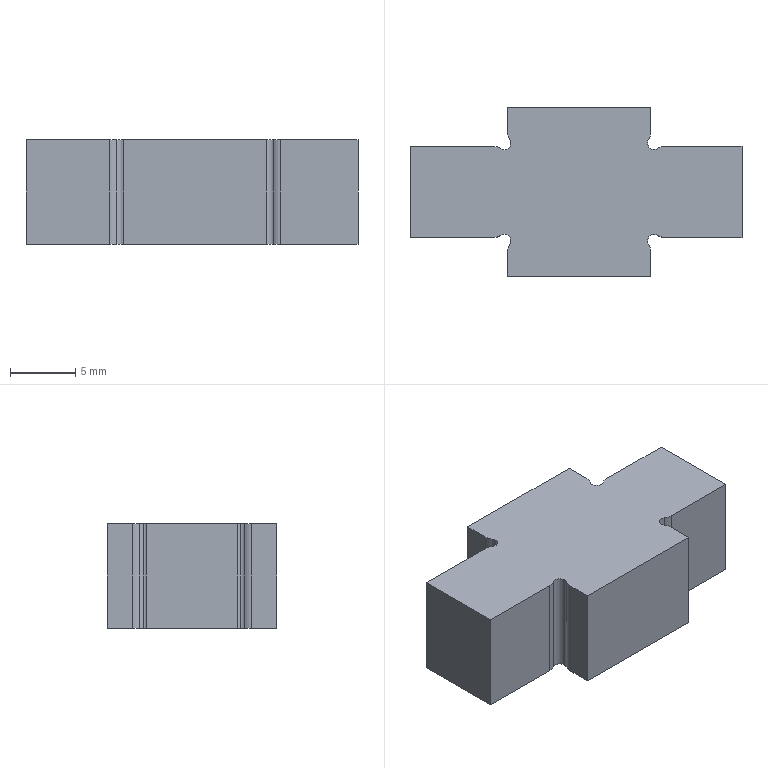Part | SolidWorks | features Fillet 1, FlatPattern 1, ICE 1, SMBaseFlange 1, SheetMetal 1 | 1 solid | 28 faces | box 25.5 x 13 x 8 mm | volume 1946 mm3 | cylinder 14 | plane 14 | commonest cylinder face diameters 2 x8 1 x6
STEP:
#1=CARTESIAN_POINT('',(-6.25,26.293,0.));
#2=VERTEX_POINT('',#1);
#3=CARTESIAN_POINT('',(-6.333,26.569,0.));
#4=VERTEX_POINT('',#3);
#5=CARTESIAN_POINT('',(-6.75,26.293,0.));
#6=DIRECTION('',(0.,0.,1.));
#7=DIRECTION('',(1.,0.,0.));
#8=AXIS2_PLACEMENT_3D('',#5,#6,#7);
#9=CIRCLE('',#8,0.5);
#10=EDGE_CURVE('',#2,#4,#9,.T.);
#11=ORIENTED_EDGE('',*,*,#10,.F.);
#12=CARTESIAN_POINT('',(-6.25,26.293,8.));
#13=VERTEX_POINT('',#12);
#14=CARTESIAN_POINT('',(-6.25,26.293,0.));
#15=DIRECTION('',(0.,0.,1.));
#16=VECTOR('',#15,1000.);
#17=LINE('',#14,#16);
#18=EDGE_CURVE('',#2,#13,#17,.T.);
#19=ORIENTED_EDGE('',*,*,#18,.T.);
#20=CARTESIAN_POINT('',(-6.333,26.569,8.));
#21=VERTEX_POINT('',#20);
#22=CARTESIAN_POINT('',(-6.75,26.293,8.));
#23=DIRECTION('',(0.,0.,1.));
#24=DIRECTION('',(1.,0.,0.));
#25=AXIS2_PLACEMENT_3D('',#22,#23,#24);
#26=CIRCLE('',#25,0.5);
#27=EDGE_CURVE('',#13,#21,#26,.T.);
#28=ORIENTED_EDGE('',*,*,#27,.T.);
#29=CARTESIAN_POINT('',(-6.333,26.569,0.));
#30=DIRECTION('',(0.,0.,-1.));
#31=VECTOR('',#30,1000.);
#32=LINE('',#29,#31);
#33=EDGE_CURVE('',#21,#4,#32,.T.);
#34=ORIENTED_EDGE('',*,*,#33,.T.);
#35=EDGE_LOOP('',(#11,#19,#28,#34));
#36=FACE_OUTER_BOUND('',#35,.T.);
#37=CARTESIAN_POINT('',(-6.75,26.293,0.));
#38=DIRECTION('',(0.,0.,1.));
#39=DIRECTION('',(1.,0.,0.));
#40=AXIS2_PLACEMENT_3D('',#37,#38,#39);
#41=CYLINDRICAL_SURFACE('',#40,0.5);
#42=ADVANCED_FACE('',(#36),#41,.F.);
#43=CARTESIAN_POINT('',(-6.25,18.793,0.));
#44=VERTEX_POINT('',#43);
#45=CARTESIAN_POINT('',(-7.026,19.209,0.));
#46=VERTEX_POINT('',#45);
#47=CARTESIAN_POINT('',(-6.75,18.793,0.));
#48=DIRECTION('',(0.,0.,1.));
#49=DIRECTION('',(1.,0.,0.));
#50=AXIS2_PLACEMENT_3D('',#47,#48,#49);
#51=CIRCLE('',#50,0.5);
#52=EDGE_CURVE('',#44,#46,#51,.T.);
#53=ORIENTED_EDGE('',*,*,#52,.F.);
#54=CARTESIAN_POINT('',(-6.25,18.793,8.));
#55=VERTEX_POINT('',#54);
#56=CARTESIAN_POINT('',(-6.25,18.793,8.));
#57=DIRECTION('',(0.,0.,1.));
#58=VECTOR('',#57,1000.);
#59=LINE('',#56,#58);
#60=EDGE_CURVE('',#44,#55,#59,.T.);
#61=ORIENTED_EDGE('',*,*,#60,.T.);
#62=CARTESIAN_POINT('',(-7.026,19.209,8.));
#63=VERTEX_POINT('',#62);
#64=CARTESIAN_POINT('',(-6.75,18.793,8.));
#65=DIRECTION('',(0.,0.,1.));
#66=DIRECTION('',(1.,0.,0.));
#67=AXIS2_PLACEMENT_3D('',#64,#65,#66);
#68=CIRCLE('',#67,0.5);
#69=EDGE_CURVE('',#55,#63,#68,.T.);
#70=ORIENTED_EDGE('',*,*,#69,.T.);
#71=CARTESIAN_POINT('',(-7.026,19.209,8.));
#72=DIRECTION('',(0.,0.,-1.));
#73=VECTOR('',#72,1000.);
#74=LINE('',#71,#73);
#75=EDGE_CURVE('',#63,#46,#74,.T.);
#76=ORIENTED_EDGE('',*,*,#75,.T.);
#77=EDGE_LOOP('',(#53,#61,#70,#76));
#78=FACE_OUTER_BOUND('',#77,.T.);
#79=CARTESIAN_POINT('',(-6.75,18.793,8.));
#80=DIRECTION('',(0.,0.,1.));
#81=DIRECTION('',(1.,0.,0.));
#82=AXIS2_PLACEMENT_3D('',#79,#80,#81);
#83=CYLINDRICAL_SURFACE('',#82,0.5);
#84=ADVANCED_FACE('',(#78),#83,.F.);
#85=CARTESIAN_POINT('',(-6.5,17.963,8.));
#86=VERTEX_POINT('',#85);
#87=CARTESIAN_POINT('',(-6.5,16.043,8.));
#88=VERTEX_POINT('',#87);
#89=CARTESIAN_POINT('',(-6.5,19.043,8.));
#90=DIRECTION('',(0.,-1.,0.));
#91=VECTOR('',#90,1000.);
#92=LINE('',#89,#91);
#93=EDGE_CURVE('',#86,#88,#92,.T.);
#94=ORIENTED_EDGE('',*,*,#93,.F.);
#95=CARTESIAN_POINT('',(-6.5,17.963,0.));
#96=VERTEX_POINT('',#95);
#97=CARTESIAN_POINT('',(-6.5,17.963,0.));
#98=DIRECTION('',(0.,0.,-1.));
#99=VECTOR('',#98,1000.);
#100=LINE('',#97,#99);
#101=EDGE_CURVE('',#86,#96,#100,.T.);
#102=ORIENTED_EDGE('',*,*,#101,.T.);
#103=CARTESIAN_POINT('',(-6.5,16.043,0.));
#104=VERTEX_POINT('',#103);
#105=CARTESIAN_POINT('',(-6.5,19.043,0.));
#106=DIRECTION('',(0.,-1.,0.));
#107=VECTOR('',#106,1000.);
#108=LINE('',#105,#107);
#109=EDGE_CURVE('',#96,#104,#108,.T.);
#110=ORIENTED_EDGE('',*,*,#109,.T.);
#111=CARTESIAN_POINT('',(-6.5,16.043,8.));
#112=DIRECTION('',(0.,0.,-1.));
#113=VECTOR('',#112,1000.);
#114=LINE('',#111,#113);
#115=EDGE_CURVE('',#88,#104,#114,.T.);
#116=ORIENTED_EDGE('',*,*,#115,.F.);
#117=EDGE_LOOP('',(#94,#102,#110,#116));
#118=FACE_OUTER_BOUND('',#117,.T.);
#119=CARTESIAN_POINT('',(-6.5,19.043,8.));
#120=DIRECTION('',(1.,0.,0.));
#121=DIRECTION('',(0.,1.,0.));
#122=AXIS2_PLACEMENT_3D('',#119,#120,#121);
#123=PLANE('',#122);
#124=ADVANCED_FACE('',(#118),#123,.F.);
#125=CARTESIAN_POINT('',(4.5,16.043,0.));
#126=VERTEX_POINT('',#125);
#127=CARTESIAN_POINT('',(4.5,17.963,0.));
#128=VERTEX_POINT('',#127);
#129=CARTESIAN_POINT('',(4.5,16.043,0.));
#130=DIRECTION('',(0.,1.,0.));
#131=VECTOR('',#130,1000.);
#132=LINE('',#129,#131);
#133=EDGE_CURVE('',#126,#128,#132,.T.);
#134=ORIENTED_EDGE('',*,*,#133,.T.);
#135=CARTESIAN_POINT('',(4.5,17.963,8.));
#136=VERTEX_POINT('',#135);
#137=CARTESIAN_POINT('',(4.5,17.963,8.));
#138=DIRECTION('',(0.,0.,1.));
#139=VECTOR('',#138,1000.);
#140=LINE('',#137,#139);
#141=EDGE_CURVE('',#128,#136,#140,.T.);
#142=ORIENTED_EDGE('',*,*,#141,.T.);
#143=CARTESIAN_POINT('',(4.5,16.043,8.));
#144=VERTEX_POINT('',#143);
#145=CARTESIAN_POINT('',(4.5,16.043,8.));
#146=DIRECTION('',(0.,1.,0.));
#147=VECTOR('',#146,1000.);
#148=LINE('',#145,#147);
#149=EDGE_CURVE('',#144,#136,#148,.T.);
#150=ORIENTED_EDGE('',*,*,#149,.F.);
#151=CARTESIAN_POINT('',(4.5,16.043,8.));
#152=DIRECTION('',(0.,0.,-1.));
#153=VECTOR('',#152,1000.);
#154=LINE('',#151,#153);
#155=EDGE_CURVE('',#144,#126,#154,.T.);
#156=ORIENTED_EDGE('',*,*,#155,.T.);
#157=EDGE_LOOP('',(#134,#142,#150,#156));
#158=FACE_OUTER_BOUND('',#157,.T.);
#159=CARTESIAN_POINT('',(4.5,16.043,8.));
#160=DIRECTION('',(-1.,0.,0.));
#161=DIRECTION('',(0.,0.,1.));
#162=AXIS2_PLACEMENT_3D('',#159,#160,#161);
#163=PLANE('',#162);
#164=ADVANCED_FACE('',(#158),#163,.F.);
#165=CARTESIAN_POINT('',(5.579,19.043,8.));
#166=VERTEX_POINT('',#165);
#167=CARTESIAN_POINT('',(11.5,19.043,8.));
#168=VERTEX_POINT('',#167);
#169=CARTESIAN_POINT('',(4.5,19.043,8.));
#170=DIRECTION('',(1.,0.,0.));
#171=VECTOR('',#170,1000.);
#172=LINE('',#169,#171);
#173=EDGE_CURVE('',#166,#168,#172,.T.);
#174=ORIENTED_EDGE('',*,*,#173,.F.);
#175=CARTESIAN_POINT('',(5.579,19.043,0.));
#176=VERTEX_POINT('',#175);
#177=CARTESIAN_POINT('',(5.579,19.043,0.));
#178=DIRECTION('',(0.,0.,-1.));
#179=VECTOR('',#178,1000.);
#180=LINE('',#177,#179);
#181=EDGE_CURVE('',#166,#176,#180,.T.);
#182=ORIENTED_EDGE('',*,*,#181,.T.);
#183=CARTESIAN_POINT('',(11.5,19.043,0.));
#184=VERTEX_POINT('',#183);
#185=CARTESIAN_POINT('',(4.5,19.043,0.));
#186=DIRECTION('',(1.,0.,0.));
#187=VECTOR('',#186,1000.);
#188=LINE('',#185,#187);
#189=EDGE_CURVE('',#176,#184,#188,.T.);
#190=ORIENTED_EDGE('',*,*,#189,.T.);
#191=CARTESIAN_POINT('',(11.5,19.043,8.));
#192=DIRECTION('',(0.,0.,-1.));
#193=VECTOR('',#192,1000.);
#194=LINE('',#191,#193);
#195=EDGE_CURVE('',#168,#184,#194,.T.);
#196=ORIENTED_EDGE('',*,*,#195,.F.);
#197=EDGE_LOOP('',(#174,#182,#190,#196));
#198=FACE_OUTER_BOUND('',#197,.T.);
#199=CARTESIAN_POINT('',(4.5,19.043,8.));
#200=DIRECTION('',(0.,1.,0.));
#201=DIRECTION('',(0.,0.,1.));
#202=AXIS2_PLACEMENT_3D('',#199,#200,#201);
#203=PLANE('',#202);
#204=ADVANCED_FACE('',(#198),#203,.F.);
#205=CARTESIAN_POINT('',(11.5,26.043,0.));
#206=VERTEX_POINT('',#205);
#207=CARTESIAN_POINT('',(5.579,26.043,0.));
#208=VERTEX_POINT('',#207);
#209=CARTESIAN_POINT('',(11.5,26.043,0.));
#210=DIRECTION('',(-1.,0.,0.));
#211=VECTOR('',#210,1000.);
#212=LINE('',#209,#211);
#213=EDGE_CURVE('',#206,#208,#212,.T.);
#214=ORIENTED_EDGE('',*,*,#213,.T.);
#215=CARTESIAN_POINT('',(5.579,26.043,8.));
#216=VERTEX_POINT('',#215);
#217=CARTESIAN_POINT('',(5.579,26.043,8.));
#218=DIRECTION('',(0.,0.,1.));
#219=VECTOR('',#218,1000.);
#220=LINE('',#217,#219);
#221=EDGE_CURVE('',#208,#216,#220,.T.);
#222=ORIENTED_EDGE('',*,*,#221,.T.);
#223=CARTESIAN_POINT('',(11.5,26.043,8.));
#224=VERTEX_POINT('',#223);
#225=CARTESIAN_POINT('',(11.5,26.043,8.));
#226=DIRECTION('',(-1.,0.,0.));
#227=VECTOR('',#226,1000.);
#228=LINE('',#225,#227);
#229=EDGE_CURVE('',#224,#216,#228,.T.);
#230=ORIENTED_EDGE('',*,*,#229,.F.);
#231=CARTESIAN_POINT('',(11.5,26.043,8.));
#232=DIRECTION('',(0.,0.,-1.));
#233=VECTOR('',#232,1000.);
#234=LINE('',#231,#233);
#235=EDGE_CURVE('',#224,#206,#234,.T.);
#236=ORIENTED_EDGE('',*,*,#235,.T.);
#237=EDGE_LOOP('',(#214,#222,#230,#236));
#238=FACE_OUTER_BOUND('',#237,.T.);
#239=CARTESIAN_POINT('',(11.5,26.043,8.));
#240=DIRECTION('',(0.,-1.,0.));
#241=DIRECTION('',(0.,0.,-1.));
#242=AXIS2_PLACEMENT_3D('',#239,#240,#241);
#243=PLANE('',#242);
#244=ADVANCED_FACE('',(#238),#243,.F.);
#245=CARTESIAN_POINT('',(4.5,27.122,8.));
#246=VERTEX_POINT('',#245);
#247=CARTESIAN_POINT('',(4.5,29.043,8.));
#248=VERTEX_POINT('',#247);
#249=CARTESIAN_POINT('',(4.5,26.043,8.));
#250=DIRECTION('',(0.,1.,0.));
#251=VECTOR('',#250,1000.);
#252=LINE('',#249,#251);
#253=EDGE_CURVE('',#246,#248,#252,.T.);
#254=ORIENTED_EDGE('',*,*,#253,.F.);
#255=CARTESIAN_POINT('',(4.5,27.122,0.));
#256=VERTEX_POINT('',#255);
#257=CARTESIAN_POINT('',(4.5,27.122,0.));
#258=DIRECTION('',(0.,0.,-1.));
#259=VECTOR('',#258,1000.);
#260=LINE('',#257,#259);
#261=EDGE_CURVE('',#246,#256,#260,.T.);
#262=ORIENTED_EDGE('',*,*,#261,.T.);
#263=CARTESIAN_POINT('',(4.5,29.043,0.));
#264=VERTEX_POINT('',#263);
#265=CARTESIAN_POINT('',(4.5,26.043,0.));
#266=DIRECTION('',(0.,1.,0.));
#267=VECTOR('',#266,1000.);
#268=LINE('',#265,#267);
#269=EDGE_CURVE('',#256,#264,#268,.T.);
#270=ORIENTED_EDGE('',*,*,#269,.T.);
#271=CARTESIAN_POINT('',(4.5,29.043,8.));
#272=DIRECTION('',(0.,0.,-1.));
#273=VECTOR('',#272,1000.);
#274=LINE('',#271,#273);
#275=EDGE_CURVE('',#248,#264,#274,.T.);
#276=ORIENTED_EDGE('',*,*,#275,.F.);
#277=EDGE_LOOP('',(#254,#262,#270,#276));
#278=FACE_OUTER_BOUND('',#277,.T.);
#279=CARTESIAN_POINT('',(4.5,26.043,8.));
#280=DIRECTION('',(-1.,0.,0.));
#281=DIRECTION('',(0.,0.,1.));
#282=AXIS2_PLACEMENT_3D('',#279,#280,#281);
#283=PLANE('',#282);
#284=ADVANCED_FACE('',(#278),#283,.F.);
#285=CARTESIAN_POINT('',(-6.5,29.043,0.));
#286=VERTEX_POINT('',#285);
#287=CARTESIAN_POINT('',(-6.5,27.122,0.));
#288=VERTEX_POINT('',#287);
#289=CARTESIAN_POINT('',(-6.5,29.043,0.));
#290=DIRECTION('',(0.,-1.,0.));
#291=VECTOR('',#290,1000.);
#292=LINE('',#289,#291);
#293=EDGE_CURVE('',#286,#288,#292,.T.);
#294=ORIENTED_EDGE('',*,*,#293,.T.);
#295=CARTESIAN_POINT('',(-6.5,27.122,8.));
#296=VERTEX_POINT('',#295);
#297=CARTESIAN_POINT('',(-6.5,27.122,8.));
#298=DIRECTION('',(0.,0.,1.));
#299=VECTOR('',#298,1000.);
#300=LINE('',#297,#299);
#301=EDGE_CURVE('',#288,#296,#300,.T.);
#302=ORIENTED_EDGE('',*,*,#301,.T.);
#303=CARTESIAN_POINT('',(-6.5,29.043,8.));
#304=VERTEX_POINT('',#303);
#305=CARTESIAN_POINT('',(-6.5,29.043,8.));
#306=DIRECTION('',(0.,-1.,0.));
#307=VECTOR('',#306,1000.);
#308=LINE('',#305,#307);
#309=EDGE_CURVE('',#304,#296,#308,.T.);
#310=ORIENTED_EDGE('',*,*,#309,.F.);
#311=CARTESIAN_POINT('',(-6.5,29.043,8.));
#312=DIRECTION('',(0.,0.,-1.));
#313=VECTOR('',#312,1000.);
#314=LINE('',#311,#313);
#315=EDGE_CURVE('',#304,#286,#314,.T.);
#316=ORIENTED_EDGE('',*,*,#315,.T.);
#317=EDGE_LOOP('',(#294,#302,#310,#316));
#318=FACE_OUTER_BOUND('',#317,.T.);
#319=CARTESIAN_POINT('',(-6.5,29.043,8.));
#320=DIRECTION('',(1.,0.,0.));
#321=DIRECTION('',(0.,0.,-1.));
#322=AXIS2_PLACEMENT_3D('',#319,#320,#321);
#323=PLANE('',#322);
#324=ADVANCED_FACE('',(#318),#323,.F.);
#325=CARTESIAN_POINT('',(-7.579,26.043,8.));
#326=VERTEX_POINT('',#325);
#327=CARTESIAN_POINT('',(-14.,26.043,8.));
#328=VERTEX_POINT('',#327);
#329=CARTESIAN_POINT('',(-14.,26.043,8.));
#330=DIRECTION('',(-1.,0.,0.));
#331=VECTOR('',#330,1000.);
#332=LINE('',#329,#331);
#333=EDGE_CURVE('',#326,#328,#332,.T.);
#334=ORIENTED_EDGE('',*,*,#333,.F.);
#335=CARTESIAN_POINT('',(-7.579,26.043,0.));
#336=VERTEX_POINT('',#335);
#337=CARTESIAN_POINT('',(-7.579,26.043,0.));
#338=DIRECTION('',(0.,0.,-1.));
#339=VECTOR('',#338,1000.);
#340=LINE('',#337,#339);
#341=EDGE_CURVE('',#326,#336,#340,.T.);
#342=ORIENTED_EDGE('',*,*,#341,.T.);
#343=CARTESIAN_POINT('',(-14.,26.043,0.));
#344=VERTEX_POINT('',#343);
#345=CARTESIAN_POINT('',(-14.,26.043,0.));
#346=DIRECTION('',(-1.,0.,0.));
#347=VECTOR('',#346,1000.);
#348=LINE('',#345,#347);
#349=EDGE_CURVE('',#336,#344,#348,.T.);
#350=ORIENTED_EDGE('',*,*,#349,.T.);
#351=CARTESIAN_POINT('',(-14.,26.043,8.));
#352=DIRECTION('',(0.,0.,-1.));
#353=VECTOR('',#352,1000.);
#354=LINE('',#351,#353);
#355=EDGE_CURVE('',#328,#344,#354,.T.);
#356=ORIENTED_EDGE('',*,*,#355,.F.);
#357=EDGE_LOOP('',(#334,#342,#350,#356));
#358=FACE_OUTER_BOUND('',#357,.T.);
#359=CARTESIAN_POINT('',(-14.,26.043,8.));
#360=DIRECTION('',(0.,-1.,0.));
#361=DIRECTION('',(0.,0.,-1.));
#362=AXIS2_PLACEMENT_3D('',#359,#360,#361);
#363=PLANE('',#362);
#364=ADVANCED_FACE('',(#358),#363,.F.);
#365=CARTESIAN_POINT('',(-14.,19.043,0.));
#366=VERTEX_POINT('',#365);
#367=CARTESIAN_POINT('',(-7.579,19.043,0.));
#368=VERTEX_POINT('',#367);
#369=CARTESIAN_POINT('',(-6.5,19.043,0.));
#370=DIRECTION('',(1.,0.,0.));
#371=VECTOR('',#370,1000.);
#372=LINE('',#369,#371);
#373=EDGE_CURVE('',#366,#368,#372,.T.);
#374=ORIENTED_EDGE('',*,*,#373,.T.);
#375=CARTESIAN_POINT('',(-7.579,19.043,8.));
#376=VERTEX_POINT('',#375);
#377=CARTESIAN_POINT('',(-7.579,19.043,8.));
#378=DIRECTION('',(0.,0.,1.));
#379=VECTOR('',#378,1000.);
#380=LINE('',#377,#379);
#381=EDGE_CURVE('',#368,#376,#380,.T.);
#382=ORIENTED_EDGE('',*,*,#381,.T.);
#383=CARTESIAN_POINT('',(-14.,19.043,8.));
#384=VERTEX_POINT('',#383);
#385=CARTESIAN_POINT('',(-6.5,19.043,8.));
#386=DIRECTION('',(1.,0.,0.));
#387=VECTOR('',#386,1000.);
#388=LINE('',#385,#387);
#389=EDGE_CURVE('',#384,#376,#388,.T.);
#390=ORIENTED_EDGE('',*,*,#389,.F.);
#391=CARTESIAN_POINT('',(-14.,19.043,8.));
#392=DIRECTION('',(0.,0.,-1.));
#393=VECTOR('',#392,1000.);
#394=LINE('',#391,#393);
#395=EDGE_CURVE('',#384,#366,#394,.T.);
#396=ORIENTED_EDGE('',*,*,#395,.T.);
#397=EDGE_LOOP('',(#374,#382,#390,#396));
#398=FACE_OUTER_BOUND('',#397,.T.);
#399=CARTESIAN_POINT('',(-6.5,19.043,8.));
#400=DIRECTION('',(0.,1.,0.));
#401=DIRECTION('',(-1.,0.,0.));
#402=AXIS2_PLACEMENT_3D('',#399,#400,#401);
#403=PLANE('',#402);
#404=ADVANCED_FACE('',(#398),#403,.F.);
#405=ORIENTED_EDGE('',*,*,#389,.T.);
#406=CARTESIAN_POINT('',(-7.579,20.043,8.));
#407=DIRECTION('',(0.,0.,1.));
#408=DIRECTION('',(1.,0.,0.));
#409=AXIS2_PLACEMENT_3D('',#406,#407,#408);
#410=CIRCLE('',#409,1.);
#411=EDGE_CURVE('',#376,#63,#410,.T.);
#412=ORIENTED_EDGE('',*,*,#411,.T.);
#413=ORIENTED_EDGE('',*,*,#69,.F.);
#414=CARTESIAN_POINT('',(-6.333,18.516,8.));
#415=VERTEX_POINT('',#414);
#416=CARTESIAN_POINT('',(-6.75,18.793,8.));
#417=DIRECTION('',(0.,0.,1.));
#418=DIRECTION('',(1.,0.,0.));
#419=AXIS2_PLACEMENT_3D('',#416,#417,#418);
#420=CIRCLE('',#419,0.5);
#421=EDGE_CURVE('',#415,#55,#420,.T.);
#422=ORIENTED_EDGE('',*,*,#421,.F.);
#423=CARTESIAN_POINT('',(-5.5,17.963,8.));
#424=DIRECTION('',(0.,0.,1.));
#425=DIRECTION('',(1.,0.,0.));
#426=AXIS2_PLACEMENT_3D('',#423,#424,#425);
#427=CIRCLE('',#426,1.);
#428=EDGE_CURVE('',#415,#86,#427,.T.);
#429=ORIENTED_EDGE('',*,*,#428,.T.);
#430=ORIENTED_EDGE('',*,*,#93,.T.);
#431=CARTESIAN_POINT('',(-6.5,16.043,8.));
#432=DIRECTION('',(1.,0.,0.));
#433=VECTOR('',#432,1000.);
#434=LINE('',#431,#433);
#435=EDGE_CURVE('',#88,#144,#434,.T.);
#436=ORIENTED_EDGE('',*,*,#435,.T.);
#437=ORIENTED_EDGE('',*,*,#149,.T.);
#438=CARTESIAN_POINT('',(4.333,18.516,8.));
#439=VERTEX_POINT('',#438);
#440=CARTESIAN_POINT('',(3.5,17.963,8.));
#441=DIRECTION('',(0.,0.,1.));
#442=DIRECTION('',(1.,0.,0.));
#443=AXIS2_PLACEMENT_3D('',#440,#441,#442);
#444=CIRCLE('',#443,1.);
#445=EDGE_CURVE('',#136,#439,#444,.T.);
#446=ORIENTED_EDGE('',*,*,#445,.T.);
#447=CARTESIAN_POINT('',(5.026,19.209,8.));
#448=VERTEX_POINT('',#447);
#449=CARTESIAN_POINT('',(4.75,18.793,8.));
#450=DIRECTION('',(0.,0.,1.));
#451=DIRECTION('',(1.,0.,0.));
#452=AXIS2_PLACEMENT_3D('',#449,#450,#451);
#453=CIRCLE('',#452,0.5);
#454=EDGE_CURVE('',#448,#439,#453,.T.);
#455=ORIENTED_EDGE('',*,*,#454,.F.);
#456=CARTESIAN_POINT('',(5.579,20.043,8.));
#457=DIRECTION('',(0.,0.,1.));
#458=DIRECTION('',(1.,0.,0.));
#459=AXIS2_PLACEMENT_3D('',#456,#457,#458);
#460=CIRCLE('',#459,1.);
#461=EDGE_CURVE('',#448,#166,#460,.T.);
#462=ORIENTED_EDGE('',*,*,#461,.T.);
#463=ORIENTED_EDGE('',*,*,#173,.T.);
#464=CARTESIAN_POINT('',(11.5,19.043,8.));
#465=DIRECTION('',(0.,1.,0.));
#466=VECTOR('',#465,1000.);
#467=LINE('',#464,#466);
#468=EDGE_CURVE('',#168,#224,#467,.T.);
#469=ORIENTED_EDGE('',*,*,#468,.T.);
#470=ORIENTED_EDGE('',*,*,#229,.T.);
#471=CARTESIAN_POINT('',(5.026,25.876,8.));
#472=VERTEX_POINT('',#471);
#473=CARTESIAN_POINT('',(5.579,25.043,8.));
#474=DIRECTION('',(0.,0.,1.));
#475=DIRECTION('',(1.,0.,0.));
#476=AXIS2_PLACEMENT_3D('',#473,#474,#475);
#477=CIRCLE('',#476,1.);
#478=EDGE_CURVE('',#216,#472,#477,.T.);
#479=ORIENTED_EDGE('',*,*,#478,.T.);
#480=CARTESIAN_POINT('',(4.333,26.569,8.));
#481=VERTEX_POINT('',#480);
#482=CARTESIAN_POINT('',(4.75,26.293,8.));
#483=DIRECTION('',(0.,0.,1.));
#484=DIRECTION('',(1.,0.,0.));
#485=AXIS2_PLACEMENT_3D('',#482,#483,#484);
#486=CIRCLE('',#485,0.5);
#487=EDGE_CURVE('',#481,#472,#486,.T.);
#488=ORIENTED_EDGE('',*,*,#487,.F.);
#489=CARTESIAN_POINT('',(3.5,27.122,8.));
#490=DIRECTION('',(0.,0.,1.));
#491=DIRECTION('',(1.,0.,0.));
#492=AXIS2_PLACEMENT_3D('',#489,#490,#491);
#493=CIRCLE('',#492,1.);
#494=EDGE_CURVE('',#481,#246,#493,.T.);
#495=ORIENTED_EDGE('',*,*,#494,.T.);
#496=ORIENTED_EDGE('',*,*,#253,.T.);
#497=CARTESIAN_POINT('',(4.5,29.043,8.));
#498=DIRECTION('',(-1.,0.,0.));
#499=VECTOR('',#498,1000.);
#500=LINE('',#497,#499);
#501=EDGE_CURVE('',#248,#304,#500,.T.);
#502=ORIENTED_EDGE('',*,*,#501,.T.);
#503=ORIENTED_EDGE('',*,*,#309,.T.);
#504=CARTESIAN_POINT('',(-5.5,27.122,8.));
#505=DIRECTION('',(0.,0.,1.));
#506=DIRECTION('',(1.,0.,0.));
#507=AXIS2_PLACEMENT_3D('',#504,#505,#506);
#508=CIRCLE('',#507,1.);
#509=EDGE_CURVE('',#296,#21,#508,.T.);
#510=ORIENTED_EDGE('',*,*,#509,.T.);
#511=ORIENTED_EDGE('',*,*,#27,.F.);
#512=CARTESIAN_POINT('',(-7.026,25.876,8.));
#513=VERTEX_POINT('',#512);
#514=CARTESIAN_POINT('',(-6.75,26.293,8.));
#515=DIRECTION('',(0.,0.,1.));
#516=DIRECTION('',(1.,0.,0.));
#517=AXIS2_PLACEMENT_3D('',#514,#515,#516);
#518=CIRCLE('',#517,0.5);
#519=EDGE_CURVE('',#513,#13,#518,.T.);
#520=ORIENTED_EDGE('',*,*,#519,.F.);
#521=CARTESIAN_POINT('',(-7.579,25.043,8.));
#522=DIRECTION('',(0.,0.,1.));
#523=DIRECTION('',(1.,0.,0.));
#524=AXIS2_PLACEMENT_3D('',#521,#522,#523);
#525=CIRCLE('',#524,1.);
#526=EDGE_CURVE('',#513,#326,#525,.T.);
#527=ORIENTED_EDGE('',*,*,#526,.T.);
#528=ORIENTED_EDGE('',*,*,#333,.T.);
#529=CARTESIAN_POINT('',(-14.,19.043,8.));
#530=DIRECTION('',(0.,-1.,0.));
#531=VECTOR('',#530,1000.);
#532=LINE('',#529,#531);
#533=EDGE_CURVE('',#328,#384,#532,.T.);
#534=ORIENTED_EDGE('',*,*,#533,.T.);
#535=EDGE_LOOP('',(#405,#412,#413,#422,#429,#430,#436,#437,#446,#455,#462,#463,#469,#470,#479,#488,#495,#496,#502,#503,#510,#511,#520,#527,#528,#534));
#536=FACE_OUTER_BOUND('',#535,.T.);
#537=CARTESIAN_POINT('',(0.,0.,8.));
#538=DIRECTION('',(0.,0.,1.));
#539=DIRECTION('',(1.,0.,0.));
#540=AXIS2_PLACEMENT_3D('',#537,#538,#539);
#541=PLANE('',#540);
#542=ADVANCED_FACE('',(#536),#541,.T.);
#543=CARTESIAN_POINT('',(-6.333,18.516,0.));
#544=VERTEX_POINT('',#543);
#545=CARTESIAN_POINT('',(-6.75,18.793,0.));
#546=DIRECTION('',(0.,0.,1.));
#547=DIRECTION('',(1.,0.,0.));
#548=AXIS2_PLACEMENT_3D('',#545,#546,#547);
#549=CIRCLE('',#548,0.5);
#550=EDGE_CURVE('',#544,#44,#549,.T.);
#551=ORIENTED_EDGE('',*,*,#550,.T.);
#552=ORIENTED_EDGE('',*,*,#52,.T.);
#553=CARTESIAN_POINT('',(-7.579,20.043,0.));
#554=DIRECTION('',(0.,0.,-1.));
#555=DIRECTION('',(1.,0.,0.));
#556=AXIS2_PLACEMENT_3D('',#553,#554,#555);
#557=CIRCLE('',#556,1.);
#558=EDGE_CURVE('',#46,#368,#557,.T.);
#559=ORIENTED_EDGE('',*,*,#558,.T.);
#560=ORIENTED_EDGE('',*,*,#373,.F.);
#561=CARTESIAN_POINT('',(-14.,19.043,0.));
#562=DIRECTION('',(0.,-1.,0.));
#563=VECTOR('',#562,1000.);
#564=LINE('',#561,#563);
#565=EDGE_CURVE('',#344,#366,#564,.T.);
#566=ORIENTED_EDGE('',*,*,#565,.F.);
#567=ORIENTED_EDGE('',*,*,#349,.F.);
#568=CARTESIAN_POINT('',(-7.026,25.876,0.));
#569=VERTEX_POINT('',#568);
#570=CARTESIAN_POINT('',(-7.579,25.043,0.));
#571=DIRECTION('',(0.,0.,-1.));
#572=DIRECTION('',(1.,0.,0.));
#573=AXIS2_PLACEMENT_3D('',#570,#571,#572);
#574=CIRCLE('',#573,1.);
#575=EDGE_CURVE('',#336,#569,#574,.T.);
#576=ORIENTED_EDGE('',*,*,#575,.T.);
#577=CARTESIAN_POINT('',(-6.75,26.293,0.));
#578=DIRECTION('',(0.,0.,1.));
#579=DIRECTION('',(1.,0.,0.));
#580=AXIS2_PLACEMENT_3D('',#577,#578,#579);
#581=CIRCLE('',#580,0.5);
#582=EDGE_CURVE('',#569,#2,#581,.T.);
#583=ORIENTED_EDGE('',*,*,#582,.T.);
#584=ORIENTED_EDGE('',*,*,#10,.T.);
#585=CARTESIAN_POINT('',(-5.5,27.122,0.));
#586=DIRECTION('',(0.,0.,-1.));
#587=DIRECTION('',(1.,0.,0.));
#588=AXIS2_PLACEMENT_3D('',#585,#586,#587);
#589=CIRCLE('',#588,1.);
#590=EDGE_CURVE('',#4,#288,#589,.T.);
#591=ORIENTED_EDGE('',*,*,#590,.T.);
#592=ORIENTED_EDGE('',*,*,#293,.F.);
#593=CARTESIAN_POINT('',(4.5,29.043,0.));
#594=DIRECTION('',(-1.,0.,0.));
#595=VECTOR('',#594,1000.);
#596=LINE('',#593,#595);
#597=EDGE_CURVE('',#264,#286,#596,.T.);
#598=ORIENTED_EDGE('',*,*,#597,.F.);
#599=ORIENTED_EDGE('',*,*,#269,.F.);
#600=CARTESIAN_POINT('',(4.333,26.569,0.));
#601=VERTEX_POINT('',#600);
#602=CARTESIAN_POINT('',(3.5,27.122,0.));
#603=DIRECTION('',(0.,0.,-1.));
#604=DIRECTION('',(1.,0.,0.));
#605=AXIS2_PLACEMENT_3D('',#602,#603,#604);
#606=CIRCLE('',#605,1.);
#607=EDGE_CURVE('',#256,#601,#606,.T.);
#608=ORIENTED_EDGE('',*,*,#607,.T.);
#609=CARTESIAN_POINT('',(5.026,25.876,0.));
#610=VERTEX_POINT('',#609);
#611=CARTESIAN_POINT('',(4.75,26.293,0.));
#612=DIRECTION('',(0.,0.,1.));
#613=DIRECTION('',(1.,0.,0.));
#614=AXIS2_PLACEMENT_3D('',#611,#612,#613);
#615=CIRCLE('',#614,0.5);
#616=EDGE_CURVE('',#601,#610,#615,.T.);
#617=ORIENTED_EDGE('',*,*,#616,.T.);
#618=CARTESIAN_POINT('',(5.579,25.043,0.));
#619=DIRECTION('',(0.,0.,-1.));
#620=DIRECTION('',(1.,0.,0.));
#621=AXIS2_PLACEMENT_3D('',#618,#619,#620);
#622=CIRCLE('',#621,1.);
#623=EDGE_CURVE('',#610,#208,#622,.T.);
#624=ORIENTED_EDGE('',*,*,#623,.T.);
#625=ORIENTED_EDGE('',*,*,#213,.F.);
#626=CARTESIAN_POINT('',(11.5,19.043,0.));
#627=DIRECTION('',(0.,1.,0.));
#628=VECTOR('',#627,1000.);
#629=LINE('',#626,#628);
#630=EDGE_CURVE('',#184,#206,#629,.T.);
#631=ORIENTED_EDGE('',*,*,#630,.F.);
#632=ORIENTED_EDGE('',*,*,#189,.F.);
#633=CARTESIAN_POINT('',(5.026,19.209,0.));
#634=VERTEX_POINT('',#633);
#635=CARTESIAN_POINT('',(5.579,20.043,0.));
#636=DIRECTION('',(0.,0.,-1.));
#637=DIRECTION('',(1.,0.,0.));
#638=AXIS2_PLACEMENT_3D('',#635,#636,#637);
#639=CIRCLE('',#638,1.);
#640=EDGE_CURVE('',#176,#634,#639,.T.);
#641=ORIENTED_EDGE('',*,*,#640,.T.);
#642=CARTESIAN_POINT('',(4.333,18.516,0.));
#643=VERTEX_POINT('',#642);
#644=CARTESIAN_POINT('',(4.75,18.793,0.));
#645=DIRECTION('',(0.,0.,1.));
#646=DIRECTION('',(1.,0.,0.));
#647=AXIS2_PLACEMENT_3D('',#644,#645,#646);
#648=CIRCLE('',#647,0.5);
#649=EDGE_CURVE('',#634,#643,#648,.T.);
#650=ORIENTED_EDGE('',*,*,#649,.T.);
#651=CARTESIAN_POINT('',(3.5,17.963,0.));
#652=DIRECTION('',(0.,0.,-1.));
#653=DIRECTION('',(1.,0.,0.));
#654=AXIS2_PLACEMENT_3D('',#651,#652,#653);
#655=CIRCLE('',#654,1.);
#656=EDGE_CURVE('',#643,#128,#655,.T.);
#657=ORIENTED_EDGE('',*,*,#656,.T.);
#658=ORIENTED_EDGE('',*,*,#133,.F.);
#659=CARTESIAN_POINT('',(-6.5,16.043,0.));
#660=DIRECTION('',(1.,0.,0.));
#661=VECTOR('',#660,1000.);
#662=LINE('',#659,#661);
#663=EDGE_CURVE('',#104,#126,#662,.T.);
#664=ORIENTED_EDGE('',*,*,#663,.F.);
#665=ORIENTED_EDGE('',*,*,#109,.F.);
#666=CARTESIAN_POINT('',(-5.5,17.963,0.));
#667=DIRECTION('',(0.,0.,-1.));
#668=DIRECTION('',(1.,0.,0.));
#669=AXIS2_PLACEMENT_3D('',#666,#667,#668);
#670=CIRCLE('',#669,1.);
#671=EDGE_CURVE('',#96,#544,#670,.T.);
#672=ORIENTED_EDGE('',*,*,#671,.T.);
#673=EDGE_LOOP('',(#551,#552,#559,#560,#566,#567,#576,#583,#584,#591,#592,#598,#599,#608,#617,#624,#625,#631,#632,#641,#650,#657,#658,#664,#665,#672));
#674=FACE_OUTER_BOUND('',#673,.T.);
#675=CARTESIAN_POINT('',(0.,0.,0.));
#676=DIRECTION('',(0.,0.,1.));
#677=DIRECTION('',(1.,0.,0.));
#678=AXIS2_PLACEMENT_3D('',#675,#676,#677);
#679=PLANE('',#678);
#680=ADVANCED_FACE('',(#674),#679,.F.);
#681=ORIENTED_EDGE('',*,*,#663,.T.);
#682=ORIENTED_EDGE('',*,*,#155,.F.);
#683=ORIENTED_EDGE('',*,*,#435,.F.);
#684=ORIENTED_EDGE('',*,*,#115,.T.);
#685=EDGE_LOOP('',(#681,#682,#683,#684));
#686=FACE_OUTER_BOUND('',#685,.T.);
#687=CARTESIAN_POINT('',(-6.5,16.043,8.));
#688=DIRECTION('',(0.,1.,0.));
#689=DIRECTION('',(-1.,0.,0.));
#690=AXIS2_PLACEMENT_3D('',#687,#688,#689);
#691=PLANE('',#690);
#692=ADVANCED_FACE('',(#686),#691,.F.);
#693=ORIENTED_EDGE('',*,*,#630,.T.);
#694=ORIENTED_EDGE('',*,*,#235,.F.);
#695=ORIENTED_EDGE('',*,*,#468,.F.);
#696=ORIENTED_EDGE('',*,*,#195,.T.);
#697=EDGE_LOOP('',(#693,#694,#695,#696));
#698=FACE_OUTER_BOUND('',#697,.T.);
#699=CARTESIAN_POINT('',(11.5,19.043,8.));
#700=DIRECTION('',(-1.,0.,0.));
#701=DIRECTION('',(0.,0.,1.));
#702=AXIS2_PLACEMENT_3D('',#699,#700,#701);
#703=PLANE('',#702);
#704=ADVANCED_FACE('',(#698),#703,.F.);
#705=ORIENTED_EDGE('',*,*,#597,.T.);
#706=ORIENTED_EDGE('',*,*,#315,.F.);
#707=ORIENTED_EDGE('',*,*,#501,.F.);
#708=ORIENTED_EDGE('',*,*,#275,.T.);
#709=EDGE_LOOP('',(#705,#706,#707,#708));
#710=FACE_OUTER_BOUND('',#709,.T.);
#711=CARTESIAN_POINT('',(4.5,29.043,8.));
#712=DIRECTION('',(0.,-1.,0.));
#713=DIRECTION('',(0.,0.,-1.));
#714=AXIS2_PLACEMENT_3D('',#711,#712,#713);
#715=PLANE('',#714);
#716=ADVANCED_FACE('',(#710),#715,.F.);
#717=ORIENTED_EDGE('',*,*,#565,.T.);
#718=ORIENTED_EDGE('',*,*,#395,.F.);
#719=ORIENTED_EDGE('',*,*,#533,.F.);
#720=ORIENTED_EDGE('',*,*,#355,.T.);
#721=EDGE_LOOP('',(#717,#718,#719,#720));
#722=FACE_OUTER_BOUND('',#721,.T.);
#723=CARTESIAN_POINT('',(-14.,19.043,8.));
#724=DIRECTION('',(1.,0.,0.));
#725=DIRECTION('',(0.,0.,-1.));
#726=AXIS2_PLACEMENT_3D('',#723,#724,#725);
#727=PLANE('',#726);
#728=ADVANCED_FACE('',(#722),#727,.F.);
#729=ORIENTED_EDGE('',*,*,#487,.T.);
#730=CARTESIAN_POINT('',(5.026,25.876,0.));
#731=DIRECTION('',(0.,0.,-1.));
#732=VECTOR('',#731,1000.);
#733=LINE('',#730,#732);
#734=EDGE_CURVE('',#472,#610,#733,.T.);
#735=ORIENTED_EDGE('',*,*,#734,.T.);
#736=ORIENTED_EDGE('',*,*,#616,.F.);
#737=CARTESIAN_POINT('',(4.333,26.569,0.));
#738=DIRECTION('',(0.,0.,1.));
#739=VECTOR('',#738,1000.);
#740=LINE('',#737,#739);
#741=EDGE_CURVE('',#601,#481,#740,.T.);
#742=ORIENTED_EDGE('',*,*,#741,.T.);
#743=EDGE_LOOP('',(#729,#735,#736,#742));
#744=FACE_OUTER_BOUND('',#743,.T.);
#745=CARTESIAN_POINT('',(4.75,26.293,0.));
#746=DIRECTION('',(0.,0.,1.));
#747=DIRECTION('',(1.,0.,0.));
#748=AXIS2_PLACEMENT_3D('',#745,#746,#747);
#749=CYLINDRICAL_SURFACE('',#748,0.5);
#750=ADVANCED_FACE('',(#744),#749,.F.);
#751=ORIENTED_EDGE('',*,*,#60,.F.);
#752=ORIENTED_EDGE('',*,*,#550,.F.);
#753=CARTESIAN_POINT('',(-6.333,18.516,8.));
#754=DIRECTION('',(0.,0.,1.));
#755=VECTOR('',#754,1000.);
#756=LINE('',#753,#755);
#757=EDGE_CURVE('',#544,#415,#756,.T.);
#758=ORIENTED_EDGE('',*,*,#757,.T.);
#759=ORIENTED_EDGE('',*,*,#421,.T.);
#760=EDGE_LOOP('',(#751,#752,#758,#759));
#761=FACE_OUTER_BOUND('',#760,.T.);
#762=CARTESIAN_POINT('',(-6.75,18.793,8.));
#763=DIRECTION('',(0.,0.,1.));
#764=DIRECTION('',(1.,0.,0.));
#765=AXIS2_PLACEMENT_3D('',#762,#763,#764);
#766=CYLINDRICAL_SURFACE('',#765,0.5);
#767=ADVANCED_FACE('',(#761),#766,.F.);
#768=ORIENTED_EDGE('',*,*,#454,.T.);
#769=CARTESIAN_POINT('',(4.333,18.516,0.));
#770=DIRECTION('',(0.,0.,-1.));
#771=VECTOR('',#770,1000.);
#772=LINE('',#769,#771);
#773=EDGE_CURVE('',#439,#643,#772,.T.);
#774=ORIENTED_EDGE('',*,*,#773,.T.);
#775=ORIENTED_EDGE('',*,*,#649,.F.);
#776=CARTESIAN_POINT('',(5.026,19.209,0.));
#777=DIRECTION('',(0.,0.,1.));
#778=VECTOR('',#777,1000.);
#779=LINE('',#776,#778);
#780=EDGE_CURVE('',#634,#448,#779,.T.);
#781=ORIENTED_EDGE('',*,*,#780,.T.);
#782=EDGE_LOOP('',(#768,#774,#775,#781));
#783=FACE_OUTER_BOUND('',#782,.T.);
#784=CARTESIAN_POINT('',(4.75,18.793,0.));
#785=DIRECTION('',(0.,0.,1.));
#786=DIRECTION('',(1.,0.,0.));
#787=AXIS2_PLACEMENT_3D('',#784,#785,#786);
#788=CYLINDRICAL_SURFACE('',#787,0.5);
#789=ADVANCED_FACE('',(#783),#788,.F.);
#790=ORIENTED_EDGE('',*,*,#18,.F.);
#791=ORIENTED_EDGE('',*,*,#582,.F.);
#792=CARTESIAN_POINT('',(-7.026,25.876,0.));
#793=DIRECTION('',(0.,0.,1.));
#794=VECTOR('',#793,1000.);
#795=LINE('',#792,#794);
#796=EDGE_CURVE('',#569,#513,#795,.T.);
#797=ORIENTED_EDGE('',*,*,#796,.T.);
#798=ORIENTED_EDGE('',*,*,#519,.T.);
#799=EDGE_LOOP('',(#790,#791,#797,#798));
#800=FACE_OUTER_BOUND('',#799,.T.);
#801=CARTESIAN_POINT('',(-6.75,26.293,0.));
#802=DIRECTION('',(0.,0.,1.));
#803=DIRECTION('',(1.,0.,0.));
#804=AXIS2_PLACEMENT_3D('',#801,#802,#803);
#805=CYLINDRICAL_SURFACE('',#804,0.5);
#806=ADVANCED_FACE('',(#800),#805,.F.);
#807=ORIENTED_EDGE('',*,*,#411,.F.);
#808=ORIENTED_EDGE('',*,*,#381,.F.);
#809=ORIENTED_EDGE('',*,*,#558,.F.);
#810=ORIENTED_EDGE('',*,*,#75,.F.);
#811=EDGE_LOOP('',(#807,#808,#809,#810));
#812=FACE_OUTER_BOUND('',#811,.T.);
#813=CARTESIAN_POINT('',(-7.579,20.043,8.));
#814=DIRECTION('',(0.,0.,1.));
#815=DIRECTION('',(1.,0.,0.));
#816=AXIS2_PLACEMENT_3D('',#813,#814,#815);
#817=CYLINDRICAL_SURFACE('',#816,1.);
#818=ADVANCED_FACE('',(#812),#817,.T.);
#819=ORIENTED_EDGE('',*,*,#428,.F.);
#820=ORIENTED_EDGE('',*,*,#757,.F.);
#821=ORIENTED_EDGE('',*,*,#671,.F.);
#822=ORIENTED_EDGE('',*,*,#101,.F.);
#823=EDGE_LOOP('',(#819,#820,#821,#822));
#824=FACE_OUTER_BOUND('',#823,.T.);
#825=CARTESIAN_POINT('',(-5.5,17.963,8.));
#826=DIRECTION('',(0.,0.,1.));
#827=DIRECTION('',(1.,0.,0.));
#828=AXIS2_PLACEMENT_3D('',#825,#826,#827);
#829=CYLINDRICAL_SURFACE('',#828,1.);
#830=ADVANCED_FACE('',(#824),#829,.T.);
#831=ORIENTED_EDGE('',*,*,#656,.F.);
#832=ORIENTED_EDGE('',*,*,#773,.F.);
#833=ORIENTED_EDGE('',*,*,#445,.F.);
#834=ORIENTED_EDGE('',*,*,#141,.F.);
#835=EDGE_LOOP('',(#831,#832,#833,#834));
#836=FACE_OUTER_BOUND('',#835,.T.);
#837=CARTESIAN_POINT('',(3.5,17.963,0.));
#838=DIRECTION('',(0.,0.,1.));
#839=DIRECTION('',(1.,0.,0.));
#840=AXIS2_PLACEMENT_3D('',#837,#838,#839);
#841=CYLINDRICAL_SURFACE('',#840,1.);
#842=ADVANCED_FACE('',(#836),#841,.T.);
#843=ORIENTED_EDGE('',*,*,#640,.F.);
#844=ORIENTED_EDGE('',*,*,#181,.F.);
#845=ORIENTED_EDGE('',*,*,#461,.F.);
#846=ORIENTED_EDGE('',*,*,#780,.F.);
#847=EDGE_LOOP('',(#843,#844,#845,#846));
#848=FACE_OUTER_BOUND('',#847,.T.);
#849=CARTESIAN_POINT('',(5.579,20.043,0.));
#850=DIRECTION('',(0.,0.,1.));
#851=DIRECTION('',(1.,0.,0.));
#852=AXIS2_PLACEMENT_3D('',#849,#850,#851);
#853=CYLINDRICAL_SURFACE('',#852,1.);
#854=ADVANCED_FACE('',(#848),#853,.T.);
#855=ORIENTED_EDGE('',*,*,#623,.F.);
#856=ORIENTED_EDGE('',*,*,#734,.F.);
#857=ORIENTED_EDGE('',*,*,#478,.F.);
#858=ORIENTED_EDGE('',*,*,#221,.F.);
#859=EDGE_LOOP('',(#855,#856,#857,#858));
#860=FACE_OUTER_BOUND('',#859,.T.);
#861=CARTESIAN_POINT('',(5.579,25.043,0.));
#862=DIRECTION('',(0.,0.,1.));
#863=DIRECTION('',(1.,0.,0.));
#864=AXIS2_PLACEMENT_3D('',#861,#862,#863);
#865=CYLINDRICAL_SURFACE('',#864,1.);
#866=ADVANCED_FACE('',(#860),#865,.T.);
#867=ORIENTED_EDGE('',*,*,#607,.F.);
#868=ORIENTED_EDGE('',*,*,#261,.F.);
#869=ORIENTED_EDGE('',*,*,#494,.F.);
#870=ORIENTED_EDGE('',*,*,#741,.F.);
#871=EDGE_LOOP('',(#867,#868,#869,#870));
#872=FACE_OUTER_BOUND('',#871,.T.);
#873=CARTESIAN_POINT('',(3.5,27.122,0.));
#874=DIRECTION('',(0.,0.,1.));
#875=DIRECTION('',(1.,0.,0.));
#876=AXIS2_PLACEMENT_3D('',#873,#874,#875);
#877=CYLINDRICAL_SURFACE('',#876,1.);
#878=ADVANCED_FACE('',(#872),#877,.T.);
#879=ORIENTED_EDGE('',*,*,#575,.F.);
#880=ORIENTED_EDGE('',*,*,#341,.F.);
#881=ORIENTED_EDGE('',*,*,#526,.F.);
#882=ORIENTED_EDGE('',*,*,#796,.F.);
#883=EDGE_LOOP('',(#879,#880,#881,#882));
#884=FACE_OUTER_BOUND('',#883,.T.);
#885=CARTESIAN_POINT('',(-7.579,25.043,0.));
#886=DIRECTION('',(0.,0.,1.));
#887=DIRECTION('',(1.,0.,0.));
#888=AXIS2_PLACEMENT_3D('',#885,#886,#887);
#889=CYLINDRICAL_SURFACE('',#888,1.);
#890=ADVANCED_FACE('',(#884),#889,.T.);
#891=ORIENTED_EDGE('',*,*,#590,.F.);
#892=ORIENTED_EDGE('',*,*,#33,.F.);
#893=ORIENTED_EDGE('',*,*,#509,.F.);
#894=ORIENTED_EDGE('',*,*,#301,.F.);
#895=EDGE_LOOP('',(#891,#892,#893,#894));
#896=FACE_OUTER_BOUND('',#895,.T.);
#897=CARTESIAN_POINT('',(-5.5,27.122,0.));
#898=DIRECTION('',(0.,0.,1.));
#899=DIRECTION('',(1.,0.,0.));
#900=AXIS2_PLACEMENT_3D('',#897,#898,#899);
#901=CYLINDRICAL_SURFACE('',#900,1.);
#902=ADVANCED_FACE('',(#896),#901,.T.);
#903=CLOSED_SHELL('',(#42,#84,#124,#164,#204,#244,#284,#324,#364,#404,#542,#680,#692,#704,#716,#728,#750,#767,#789,#806,#818,#830,#842,#854,#866,#878,#890,#902));
#904=MANIFOLD_SOLID_BREP('',#903);
#905=CARTESIAN_POINT('',(0.,0.,0.));
#906=DIRECTION('',(0.,0.,1.));
#907=DIRECTION('',(1.,0.,0.));
#908=AXIS2_PLACEMENT_3D('',#905,#906,#907);
#909=(LENGTH_UNIT()NAMED_UNIT(*)SI_UNIT(.MILLI.,.METRE.));
#910=UNCERTAINTY_MEASURE_WITH_UNIT(LENGTH_MEASURE(0.00001),#909,'','');
#911=(NAMED_UNIT(*)PLANE_ANGLE_UNIT()SI_UNIT($,.RADIAN.));
#912=(NAMED_UNIT(*)SI_UNIT($,.STERADIAN.)SOLID_ANGLE_UNIT());
#913=(GEOMETRIC_REPRESENTATION_CONTEXT(3)GLOBAL_UNCERTAINTY_ASSIGNED_CONTEXT((#910))GLOBAL_UNIT_ASSIGNED_CONTEXT((#909,#911,#912))REPRESENTATION_CONTEXT('',''));
#914=ADVANCED_BREP_SHAPE_REPRESENTATION('',(#904,#908),#913);